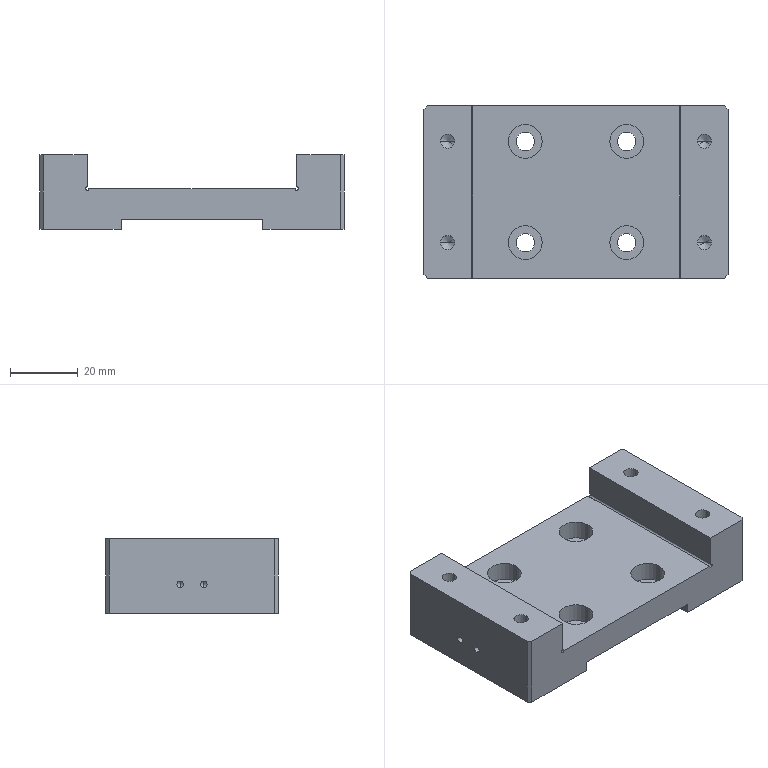Part | STEP file | ASND-0110-TCTF01-31 | 1 solid | 66 faces | box 90 x 51 x 22 mm | volume 59920 mm3 | cylinder 32 | plane 22 | cone 12 | commonest cylinder face diameters 4.2 x8 5.5 x8 10 x8 1 x4 2 x4